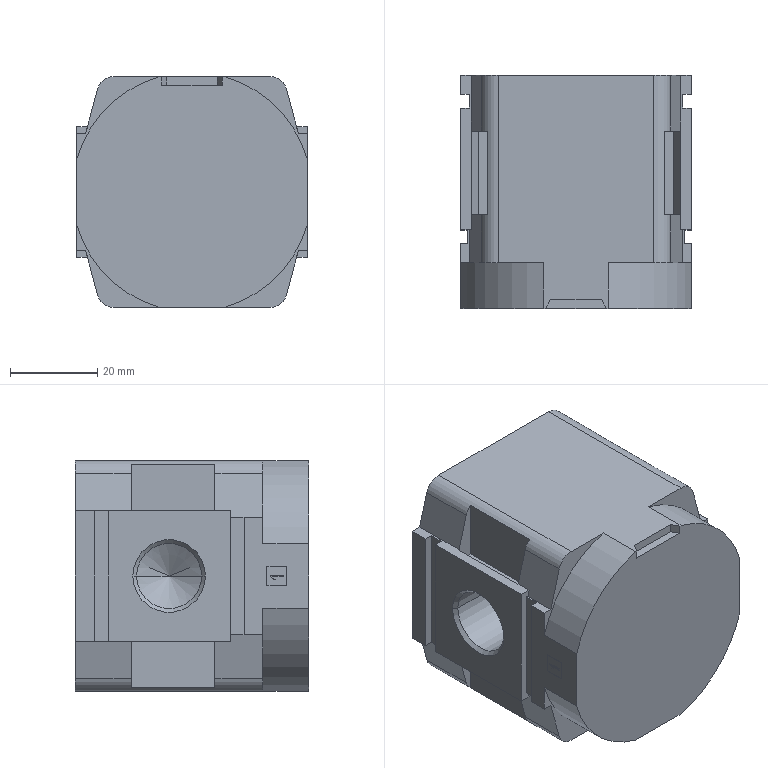Part | SolidWorks | features BaseBody 1 | 1 solid | 162 faces | box 53 x 53.5 x 53 mm | volume 128683 mm3 | plane 126 | cylinder 28 | cone 8 | commonest cylinder face diameters 8 x4 14.95 x4 55 x4 1.132 x2 1.336 x2 0.742 x1